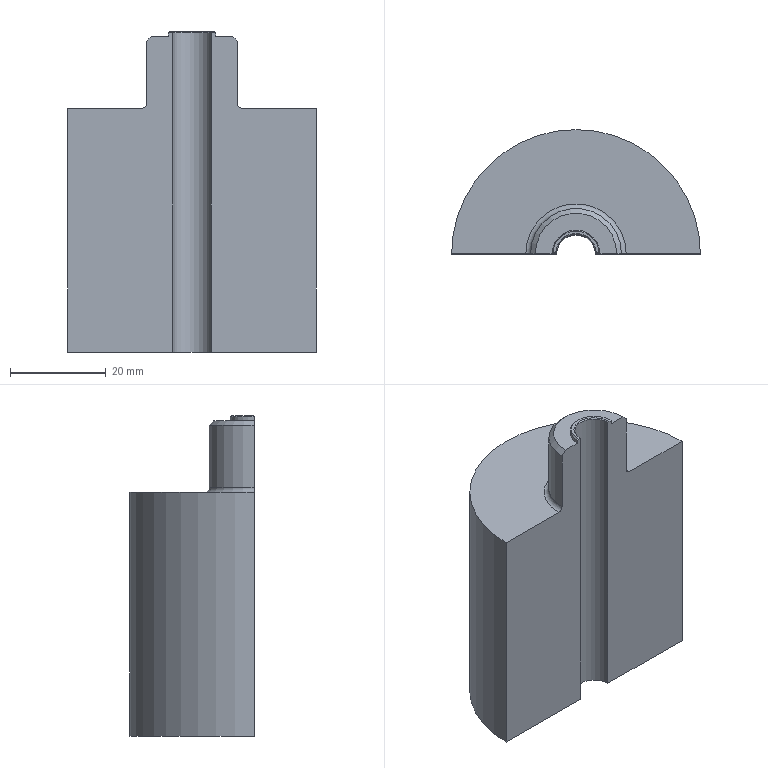Part | STEP file | 001-009-Riveting mechanism lower die insert | 1 solid | 16 faces | box 52 x 26 x 67 mm | volume 54586 mm3 | plane 8 | cylinder 4 | cone 3 | torus 1 | commonest cylinder face diameters 8.1 x1 10 x1 19 x1 52 x1
STEP:
#1=CARTESIAN_POINT('',(0.,0.,0.));
#2=DIRECTION('',(0.,0.,1.));
#3=DIRECTION('',(1.,0.,0.));
#4=AXIS2_PLACEMENT_3D('',#1,#2,#3);
#5=CARTESIAN_POINT('',(-5.,0.,66.));
#6=VERTEX_POINT('',#5);
#7=CARTESIAN_POINT('',(-8.5,0.,66.));
#8=VERTEX_POINT('',#7);
#9=CARTESIAN_POINT('',(0.,0.,66.));
#10=DIRECTION('',(-1.,0.,0.));
#11=VECTOR('',#10,1.);
#12=LINE('',#9,#11);
#13=CARTESIAN_POINT('',(0.,0.,0.));
#14=DIRECTION('',(0.,1.,0.));
#15=DIRECTION('',(0.,0.,1.));
#16=AXIS2_PLACEMENT_3D('',#13,#14,#15);
#17=PLANE('',#16);
#18=CARTESIAN_POINT('',(66.,0.));
#19=DIRECTION('',(0.,-1.));
#20=VECTOR('',#19,1.);
#21=LINE('',#18,#20);
#22=(GEOMETRIC_REPRESENTATION_CONTEXT(2)PARAMETRIC_REPRESENTATION_CONTEXT()REPRESENTATION_CONTEXT('',''));
#23=DEFINITIONAL_REPRESENTATION('',(#21),#22);
#24=PCURVE('',#17,#23);
#25=CARTESIAN_POINT('',(0.,0.,66.));
#26=DIRECTION('',(0.,0.,1.));
#27=DIRECTION('',(1.,0.,0.));
#28=AXIS2_PLACEMENT_3D('',#25,#26,#27);
#29=PLANE('',#28);
#30=CARTESIAN_POINT('',(0.,0.));
#31=DIRECTION('',(-1.,0.));
#32=VECTOR('',#31,1.);
#33=LINE('',#30,#32);
#34=(GEOMETRIC_REPRESENTATION_CONTEXT(2)PARAMETRIC_REPRESENTATION_CONTEXT()REPRESENTATION_CONTEXT('',''));
#35=DEFINITIONAL_REPRESENTATION('',(#33),#34);
#36=PCURVE('',#29,#35);
#37=SURFACE_CURVE('',#12,(#24,#36),.PCURVE_S1.);
#38=EDGE_CURVE('',#6,#8,#37,.T.);
#39=ORIENTED_EDGE('',*,*,#38,.T.);
#40=CARTESIAN_POINT('',(-9.5,0.,65.));
#41=VERTEX_POINT('',#40);
#42=CARTESIAN_POINT('',(0.,0.,74.5));
#43=DIRECTION('',(-0.7071,0.,-0.7071));
#44=VECTOR('',#43,1.);
#45=LINE('',#42,#44);
#46=CARTESIAN_POINT('',(74.5,0.));
#47=DIRECTION('',(-0.7071,-0.7071));
#48=VECTOR('',#47,1.);
#49=LINE('',#46,#48);
#50=(GEOMETRIC_REPRESENTATION_CONTEXT(2)PARAMETRIC_REPRESENTATION_CONTEXT()REPRESENTATION_CONTEXT('',''));
#51=DEFINITIONAL_REPRESENTATION('',(#49),#50);
#52=PCURVE('',#17,#51);
#53=CARTESIAN_POINT('',(0.,0.,66.));
#54=DIRECTION('',(0.,0.,-1.));
#55=DIRECTION('',(-1.,0.,0.));
#56=AXIS2_PLACEMENT_3D('',#53,#54,#55);
#57=CONICAL_SURFACE('',#56,8.5,0.7854);
#58=CARTESIAN_POINT('',(0.,-8.5));
#59=DIRECTION('',(0.,1.));
#60=VECTOR('',#59,1.);
#61=LINE('',#58,#60);
#62=(GEOMETRIC_REPRESENTATION_CONTEXT(2)PARAMETRIC_REPRESENTATION_CONTEXT()REPRESENTATION_CONTEXT('',''));
#63=DEFINITIONAL_REPRESENTATION('',(#61),#62);
#64=PCURVE('',#57,#63);
#65=SURFACE_CURVE('',#45,(#52,#64),.PCURVE_S1.);
#66=EDGE_CURVE('',#8,#41,#65,.T.);
#67=ORIENTED_EDGE('',*,*,#66,.T.);
#68=CARTESIAN_POINT('',(-9.5,0.,52.));
#69=VERTEX_POINT('',#68);
#70=CARTESIAN_POINT('',(-9.5,0.,67.));
#71=DIRECTION('',(0.,0.,1.));
#72=VECTOR('',#71,1.);
#73=LINE('',#70,#72);
#74=CARTESIAN_POINT('',(67.,-9.5));
#75=DIRECTION('',(1.,0.));
#76=VECTOR('',#75,1.);
#77=LINE('',#74,#76);
#78=(GEOMETRIC_REPRESENTATION_CONTEXT(2)PARAMETRIC_REPRESENTATION_CONTEXT()REPRESENTATION_CONTEXT('',''));
#79=DEFINITIONAL_REPRESENTATION('',(#77),#78);
#80=PCURVE('',#17,#79);
#81=CARTESIAN_POINT('',(0.,0.,67.));
#82=DIRECTION('',(0.,0.,-1.));
#83=DIRECTION('',(-1.,0.,0.));
#84=AXIS2_PLACEMENT_3D('',#81,#82,#83);
#85=CYLINDRICAL_SURFACE('',#84,9.5);
#86=CARTESIAN_POINT('',(0.,0.));
#87=DIRECTION('',(0.,-1.));
#88=VECTOR('',#87,1.);
#89=LINE('',#86,#88);
#90=(GEOMETRIC_REPRESENTATION_CONTEXT(2)PARAMETRIC_REPRESENTATION_CONTEXT()REPRESENTATION_CONTEXT('',''));
#91=DEFINITIONAL_REPRESENTATION('',(#89),#90);
#92=PCURVE('',#85,#91);
#93=SURFACE_CURVE('',#73,(#80,#92),.PCURVE_S1.);
#94=EDGE_CURVE('',#69,#41,#93,.T.);
#95=ORIENTED_EDGE('',*,*,#94,.F.);
#96=CARTESIAN_POINT('',(-10.5,0.,51.));
#97=VERTEX_POINT('',#96);
#98=CARTESIAN_POINT('',(-10.5,0.,52.));
#99=DIRECTION('',(0.,1.,0.));
#100=DIRECTION('',(0.,0.,1.));
#101=AXIS2_PLACEMENT_3D('',#98,#99,#100);
#102=CIRCLE('',#101,1.);
#103=CARTESIAN_POINT('',(52.,-10.5));
#104=DIRECTION('',(1.,0.));
#105=AXIS2_PLACEMENT_2D('',#103,#104);
#106=CIRCLE('',#105,1.);
#107=(GEOMETRIC_REPRESENTATION_CONTEXT(2)PARAMETRIC_REPRESENTATION_CONTEXT()REPRESENTATION_CONTEXT('',''));
#108=DEFINITIONAL_REPRESENTATION('',(#106),#107);
#109=PCURVE('',#17,#108);
#110=CARTESIAN_POINT('',(0.,0.,52.));
#111=DIRECTION('',(0.,0.,1.));
#112=DIRECTION('',(1.,0.,0.));
#113=AXIS2_PLACEMENT_3D('',#110,#111,#112);
#114=TOROIDAL_SURFACE('',#113,10.5,1.);
#115=CARTESIAN_POINT('',(3.142,1.571));
#116=DIRECTION('',(0.,1.));
#117=VECTOR('',#116,1.);
#118=LINE('',#115,#117);
#119=(GEOMETRIC_REPRESENTATION_CONTEXT(2)PARAMETRIC_REPRESENTATION_CONTEXT()REPRESENTATION_CONTEXT('',''));
#120=DEFINITIONAL_REPRESENTATION('',(#118),#119);
#121=PCURVE('',#114,#120);
#122=SURFACE_CURVE('',#102,(#109,#121),.PCURVE_S1.);
#123=EDGE_CURVE('',#69,#97,#122,.T.);
#124=ORIENTED_EDGE('',*,*,#123,.T.);
#125=CARTESIAN_POINT('',(-26.,0.,51.));
#126=VERTEX_POINT('',#125);
#127=CARTESIAN_POINT('',(0.,0.,51.));
#128=DIRECTION('',(-1.,0.,0.));
#129=VECTOR('',#128,1.);
#130=LINE('',#127,#129);
#131=CARTESIAN_POINT('',(51.,0.));
#132=DIRECTION('',(0.,-1.));
#133=VECTOR('',#132,1.);
#134=LINE('',#131,#133);
#135=(GEOMETRIC_REPRESENTATION_CONTEXT(2)PARAMETRIC_REPRESENTATION_CONTEXT()REPRESENTATION_CONTEXT('',''));
#136=DEFINITIONAL_REPRESENTATION('',(#134),#135);
#137=PCURVE('',#17,#136);
#138=CARTESIAN_POINT('',(0.,0.,51.));
#139=DIRECTION('',(0.,0.,1.));
#140=DIRECTION('',(1.,0.,0.));
#141=AXIS2_PLACEMENT_3D('',#138,#139,#140);
#142=PLANE('',#141);
#143=CARTESIAN_POINT('',(0.,0.));
#144=DIRECTION('',(-1.,0.));
#145=VECTOR('',#144,1.);
#146=LINE('',#143,#145);
#147=(GEOMETRIC_REPRESENTATION_CONTEXT(2)PARAMETRIC_REPRESENTATION_CONTEXT()REPRESENTATION_CONTEXT('',''));
#148=DEFINITIONAL_REPRESENTATION('',(#146),#147);
#149=PCURVE('',#142,#148);
#150=SURFACE_CURVE('',#130,(#137,#149),.PCURVE_S1.);
#151=EDGE_CURVE('',#97,#126,#150,.T.);
#152=ORIENTED_EDGE('',*,*,#151,.T.);
#153=CARTESIAN_POINT('',(-26.,0.,0.));
#154=VERTEX_POINT('',#153);
#155=CARTESIAN_POINT('',(-26.,0.,51.));
#156=DIRECTION('',(0.,0.,1.));
#157=VECTOR('',#156,1.);
#158=LINE('',#155,#157);
#159=CARTESIAN_POINT('',(51.,-26.));
#160=DIRECTION('',(1.,0.));
#161=VECTOR('',#160,1.);
#162=LINE('',#159,#161);
#163=(GEOMETRIC_REPRESENTATION_CONTEXT(2)PARAMETRIC_REPRESENTATION_CONTEXT()REPRESENTATION_CONTEXT('',''));
#164=DEFINITIONAL_REPRESENTATION('',(#162),#163);
#165=PCURVE('',#17,#164);
#166=CARTESIAN_POINT('',(0.,0.,51.));
#167=DIRECTION('',(0.,0.,-1.));
#168=DIRECTION('',(-1.,0.,0.));
#169=AXIS2_PLACEMENT_3D('',#166,#167,#168);
#170=CYLINDRICAL_SURFACE('',#169,26.);
#171=CARTESIAN_POINT('',(0.,0.));
#172=DIRECTION('',(0.,-1.));
#173=VECTOR('',#172,1.);
#174=LINE('',#171,#173);
#175=(GEOMETRIC_REPRESENTATION_CONTEXT(2)PARAMETRIC_REPRESENTATION_CONTEXT()REPRESENTATION_CONTEXT('',''));
#176=DEFINITIONAL_REPRESENTATION('',(#174),#175);
#177=PCURVE('',#170,#176);
#178=SURFACE_CURVE('',#158,(#165,#177),.PCURVE_S1.);
#179=EDGE_CURVE('',#154,#126,#178,.T.);
#180=ORIENTED_EDGE('',*,*,#179,.F.);
#181=CARTESIAN_POINT('',(-4.05,0.,0.));
#182=VERTEX_POINT('',#181);
#183=CARTESIAN_POINT('',(0.,0.,0.));
#184=DIRECTION('',(-1.,0.,0.));
#185=VECTOR('',#184,1.);
#186=LINE('',#183,#185);
#187=CARTESIAN_POINT('',(0.,0.));
#188=DIRECTION('',(0.,-1.));
#189=VECTOR('',#188,1.);
#190=LINE('',#187,#189);
#191=(GEOMETRIC_REPRESENTATION_CONTEXT(2)PARAMETRIC_REPRESENTATION_CONTEXT()REPRESENTATION_CONTEXT('',''));
#192=DEFINITIONAL_REPRESENTATION('',(#190),#191);
#193=PCURVE('',#17,#192);
#194=CARTESIAN_POINT('',(0.,0.,0.));
#195=DIRECTION('',(0.,0.,1.));
#196=DIRECTION('',(1.,0.,0.));
#197=AXIS2_PLACEMENT_3D('',#194,#195,#196);
#198=PLANE('',#197);
#199=CARTESIAN_POINT('',(0.,0.));
#200=DIRECTION('',(-1.,0.));
#201=VECTOR('',#200,1.);
#202=LINE('',#199,#201);
#203=(GEOMETRIC_REPRESENTATION_CONTEXT(2)PARAMETRIC_REPRESENTATION_CONTEXT()REPRESENTATION_CONTEXT('',''));
#204=DEFINITIONAL_REPRESENTATION('',(#202),#203);
#205=PCURVE('',#198,#204);
#206=SURFACE_CURVE('',#186,(#193,#205),.PCURVE_S1.);
#207=EDGE_CURVE('',#182,#154,#206,.T.);
#208=ORIENTED_EDGE('',*,*,#207,.F.);
#209=CARTESIAN_POINT('',(-4.05,0.,66.8));
#210=VERTEX_POINT('',#209);
#211=CARTESIAN_POINT('',(-4.05,0.,0.));
#212=DIRECTION('',(0.,0.,-1.));
#213=VECTOR('',#212,1.);
#214=LINE('',#211,#213);
#215=CARTESIAN_POINT('',(0.,-4.05));
#216=DIRECTION('',(-1.,0.));
#217=VECTOR('',#216,1.);
#218=LINE('',#215,#217);
#219=(GEOMETRIC_REPRESENTATION_CONTEXT(2)PARAMETRIC_REPRESENTATION_CONTEXT()REPRESENTATION_CONTEXT('',''));
#220=DEFINITIONAL_REPRESENTATION('',(#218),#219);
#221=PCURVE('',#17,#220);
#222=CARTESIAN_POINT('',(0.,0.,0.));
#223=DIRECTION('',(0.,0.,1.));
#224=DIRECTION('',(1.,0.,0.));
#225=AXIS2_PLACEMENT_3D('',#222,#223,#224);
#226=CYLINDRICAL_SURFACE('',#225,4.05);
#227=CARTESIAN_POINT('',(3.142,0.));
#228=DIRECTION('',(0.,-1.));
#229=VECTOR('',#228,1.);
#230=LINE('',#227,#229);
#231=(GEOMETRIC_REPRESENTATION_CONTEXT(2)PARAMETRIC_REPRESENTATION_CONTEXT()REPRESENTATION_CONTEXT('',''));
#232=DEFINITIONAL_REPRESENTATION('',(#230),#231);
#233=PCURVE('',#226,#232);
#234=SURFACE_CURVE('',#214,(#221,#233),.PCURVE_S1.);
#235=EDGE_CURVE('',#210,#182,#234,.T.);
#236=ORIENTED_EDGE('',*,*,#235,.F.);
#237=CARTESIAN_POINT('',(-5.,0.,66.8));
#238=VERTEX_POINT('',#237);
#239=CARTESIAN_POINT('',(-5.,0.,66.8));
#240=DIRECTION('',(-1.,0.,0.));
#241=VECTOR('',#240,1.);
#242=LINE('',#239,#241);
#243=CARTESIAN_POINT('',(66.8,-5.));
#244=DIRECTION('',(0.,-1.));
#245=VECTOR('',#244,1.);
#246=LINE('',#243,#245);
#247=(GEOMETRIC_REPRESENTATION_CONTEXT(2)PARAMETRIC_REPRESENTATION_CONTEXT()REPRESENTATION_CONTEXT('',''));
#248=DEFINITIONAL_REPRESENTATION('',(#246),#247);
#249=PCURVE('',#17,#248);
#250=CARTESIAN_POINT('',(0.,0.,66.8));
#251=DIRECTION('',(0.,-0.7071,0.7071));
#252=DIRECTION('',(1.,0.,0.));
#253=AXIS2_PLACEMENT_3D('',#250,#251,#252);
#254=PLANE('',#253);
#255=CARTESIAN_POINT('',(-5.,0.));
#256=DIRECTION('',(-1.,0.));
#257=VECTOR('',#256,1.);
#258=LINE('',#255,#257);
#259=(GEOMETRIC_REPRESENTATION_CONTEXT(2)PARAMETRIC_REPRESENTATION_CONTEXT()REPRESENTATION_CONTEXT('',''));
#260=DEFINITIONAL_REPRESENTATION('',(#258),#259);
#261=PCURVE('',#254,#260);
#262=SURFACE_CURVE('',#242,(#249,#261),.PCURVE_S1.);
#263=EDGE_CURVE('',#210,#238,#262,.T.);
#264=ORIENTED_EDGE('',*,*,#263,.T.);
#265=CARTESIAN_POINT('',(-5.,0.,66.));
#266=DIRECTION('',(0.,0.,-1.));
#267=VECTOR('',#266,1.);
#268=LINE('',#265,#267);
#269=CARTESIAN_POINT('',(66.,-5.));
#270=DIRECTION('',(-1.,0.));
#271=VECTOR('',#270,1.);
#272=LINE('',#269,#271);
#273=(GEOMETRIC_REPRESENTATION_CONTEXT(2)PARAMETRIC_REPRESENTATION_CONTEXT()REPRESENTATION_CONTEXT('',''));
#274=DEFINITIONAL_REPRESENTATION('',(#272),#273);
#275=PCURVE('',#17,#274);
#276=CARTESIAN_POINT('',(0.,0.,66.));
#277=DIRECTION('',(0.,0.,1.));
#278=DIRECTION('',(1.,0.,0.));
#279=AXIS2_PLACEMENT_3D('',#276,#277,#278);
#280=CYLINDRICAL_SURFACE('',#279,5.);
#281=CARTESIAN_POINT('',(3.142,0.));
#282=DIRECTION('',(0.,-1.));
#283=VECTOR('',#282,1.);
#284=LINE('',#281,#283);
#285=(GEOMETRIC_REPRESENTATION_CONTEXT(2)PARAMETRIC_REPRESENTATION_CONTEXT()REPRESENTATION_CONTEXT('',''));
#286=DEFINITIONAL_REPRESENTATION('',(#284),#285);
#287=PCURVE('',#280,#286);
#288=SURFACE_CURVE('',#268,(#275,#287),.PCURVE_S1.);
#289=EDGE_CURVE('',#238,#6,#288,.T.);
#290=ORIENTED_EDGE('',*,*,#289,.T.);
#291=EDGE_LOOP('',(#39,#67,#95,#124,#152,#180,#208,#236,#264,#290));
#292=FACE_BOUND('',#291,.T.);
#293=ADVANCED_FACE('',(#292),#17,.F.);
#294=ORIENTED_EDGE('',*,*,#94,.T.);
#295=CARTESIAN_POINT('',(9.5,0.,65.));
#296=VERTEX_POINT('',#295);
#297=CARTESIAN_POINT('',(0.,0.,65.));
#298=DIRECTION('',(0.,0.,-1.));
#299=DIRECTION('',(1.,0.,0.));
#300=AXIS2_PLACEMENT_3D('',#297,#298,#299);
#301=CIRCLE('',#300,9.5);
#302=CARTESIAN_POINT('',(-3.142,2.));
#303=DIRECTION('',(1.,0.));
#304=VECTOR('',#303,1.);
#305=LINE('',#302,#304);
#306=(GEOMETRIC_REPRESENTATION_CONTEXT(2)PARAMETRIC_REPRESENTATION_CONTEXT()REPRESENTATION_CONTEXT('',''));
#307=DEFINITIONAL_REPRESENTATION('',(#305),#306);
#308=PCURVE('',#85,#307);
#309=CARTESIAN_POINT('',(-3.142,1.));
#310=DIRECTION('',(1.,0.));
#311=VECTOR('',#310,1.);
#312=LINE('',#309,#311);
#313=(GEOMETRIC_REPRESENTATION_CONTEXT(2)PARAMETRIC_REPRESENTATION_CONTEXT()REPRESENTATION_CONTEXT('',''));
#314=DEFINITIONAL_REPRESENTATION('',(#312),#313);
#315=PCURVE('',#57,#314);
#316=SURFACE_CURVE('',#301,(#308,#315),.PCURVE_S1.);
#317=EDGE_CURVE('',#41,#296,#316,.T.);
#318=ORIENTED_EDGE('',*,*,#317,.T.);
#319=CARTESIAN_POINT('',(9.5,0.,52.));
#320=VERTEX_POINT('',#319);
#321=CARTESIAN_POINT('',(9.5,0.,67.));
#322=DIRECTION('',(0.,0.,-1.));
#323=VECTOR('',#322,1.);
#324=LINE('',#321,#323);
#325=CARTESIAN_POINT('',(3.142,0.));
#326=DIRECTION('',(0.,1.));
#327=VECTOR('',#326,1.);
#328=LINE('',#325,#327);
#329=(GEOMETRIC_REPRESENTATION_CONTEXT(2)PARAMETRIC_REPRESENTATION_CONTEXT()REPRESENTATION_CONTEXT('',''));
#330=DEFINITIONAL_REPRESENTATION('',(#328),#329);
#331=PCURVE('',#85,#330);
#332=CARTESIAN_POINT('',(0.,0.,0.));
#333=DIRECTION('',(0.,1.,0.));
#334=DIRECTION('',(0.,0.,1.));
#335=AXIS2_PLACEMENT_3D('',#332,#333,#334);
#336=PLANE('',#335);
#337=CARTESIAN_POINT('',(67.,9.5));
#338=DIRECTION('',(-1.,0.));
#339=VECTOR('',#338,1.);
#340=LINE('',#337,#339);
#341=(GEOMETRIC_REPRESENTATION_CONTEXT(2)PARAMETRIC_REPRESENTATION_CONTEXT()REPRESENTATION_CONTEXT('',''));
#342=DEFINITIONAL_REPRESENTATION('',(#340),#341);
#343=PCURVE('',#336,#342);
#344=SURFACE_CURVE('',#324,(#331,#343),.PCURVE_S1.);
#345=EDGE_CURVE('',#296,#320,#344,.T.);
#346=ORIENTED_EDGE('',*,*,#345,.T.);
#347=CARTESIAN_POINT('',(0.,0.,52.));
#348=DIRECTION('',(0.,0.,1.));
#349=DIRECTION('',(1.,0.,0.));
#350=AXIS2_PLACEMENT_3D('',#347,#348,#349);
#351=CIRCLE('',#350,9.5);
#352=CARTESIAN_POINT('',(3.142,15.));
#353=DIRECTION('',(-1.,0.));
#354=VECTOR('',#353,1.);
#355=LINE('',#352,#354);
#356=(GEOMETRIC_REPRESENTATION_CONTEXT(2)PARAMETRIC_REPRESENTATION_CONTEXT()REPRESENTATION_CONTEXT('',''));
#357=DEFINITIONAL_REPRESENTATION('',(#355),#356);
#358=PCURVE('',#85,#357);
#359=CARTESIAN_POINT('',(0.,3.142));
#360=DIRECTION('',(1.,0.));
#361=VECTOR('',#360,1.);
#362=LINE('',#359,#361);
#363=(GEOMETRIC_REPRESENTATION_CONTEXT(2)PARAMETRIC_REPRESENTATION_CONTEXT()REPRESENTATION_CONTEXT('',''));
#364=DEFINITIONAL_REPRESENTATION('',(#362),#363);
#365=PCURVE('',#114,#364);
#366=SURFACE_CURVE('',#351,(#358,#365),.PCURVE_S1.);
#367=EDGE_CURVE('',#320,#69,#366,.T.);
#368=ORIENTED_EDGE('',*,*,#367,.T.);
#369=EDGE_LOOP('',(#294,#318,#346,#368));
#370=FACE_BOUND('',#369,.T.);
#371=ADVANCED_FACE('',(#370),#85,.T.);
#372=CARTESIAN_POINT('',(-4.796,0.2,67.));
#373=VERTEX_POINT('',#372);
#374=CARTESIAN_POINT('',(-4.245,0.2,67.));
#375=VERTEX_POINT('',#374);
#376=CARTESIAN_POINT('',(-4.05,0.2,67.));
#377=DIRECTION('',(1.,0.,0.));
#378=VECTOR('',#377,1.);
#379=LINE('',#376,#378);
#380=CARTESIAN_POINT('',(0.,0.,67.));
#381=DIRECTION('',(0.,0.,1.));
#382=DIRECTION('',(1.,0.,0.));
#383=AXIS2_PLACEMENT_3D('',#380,#381,#382);
#384=PLANE('',#383);
#385=CARTESIAN_POINT('',(-4.05,0.2));
#386=DIRECTION('',(1.,0.));
#387=VECTOR('',#386,1.);
#388=LINE('',#385,#387);
#389=(GEOMETRIC_REPRESENTATION_CONTEXT(2)PARAMETRIC_REPRESENTATION_CONTEXT()REPRESENTATION_CONTEXT('',''));
#390=DEFINITIONAL_REPRESENTATION('',(#388),#389);
#391=PCURVE('',#384,#390);
#392=CARTESIAN_POINT('',(-4.05,0.2828));
#393=DIRECTION('',(1.,0.));
#394=VECTOR('',#393,1.);
#395=LINE('',#392,#394);
#396=(GEOMETRIC_REPRESENTATION_CONTEXT(2)PARAMETRIC_REPRESENTATION_CONTEXT()REPRESENTATION_CONTEXT('',''));
#397=DEFINITIONAL_REPRESENTATION('',(#395),#396);
#398=PCURVE('',#254,#397);
#399=SURFACE_CURVE('',#379,(#391,#398),.PCURVE_S1.);
#400=EDGE_CURVE('',#373,#375,#399,.T.);
#401=ORIENTED_EDGE('',*,*,#400,.T.);
#402=CARTESIAN_POINT('',(4.245,0.2,67.));
#403=VERTEX_POINT('',#402);
#404=CARTESIAN_POINT('',(0.,0.,67.));
#405=DIRECTION('',(0.,0.,-1.));
#406=DIRECTION('',(1.,0.,0.));
#407=AXIS2_PLACEMENT_3D('',#404,#405,#406);
#408=CIRCLE('',#407,4.25);
#409=CARTESIAN_POINT('',(4.25,0.));
#410=CARTESIAN_POINT('',(4.25,-7.361));
#411=CARTESIAN_POINT('',(-2.125,-3.681));
#412=CARTESIAN_POINT('',(-8.5,0.));
#413=CARTESIAN_POINT('',(-2.125,3.681));
#414=CARTESIAN_POINT('',(4.25,7.361));
#415=CARTESIAN_POINT('',(4.25,0.));
#416=(BOUNDED_CURVE()B_SPLINE_CURVE(2,(#409,#410,#411,#412,#413,#414,#415),.UNSPECIFIED.,.T.,.F.)B_SPLINE_CURVE_WITH_KNOTS((1,2,2,2,2,1),(-2.094,0.,2.094,4.189,6.283,8.378),.UNSPECIFIED.)CURVE()GEOMETRIC_REPRESENTATION_ITEM()RATIONAL_B_SPLINE_CURVE((1.,0.5,1.,0.5,1.,0.5,1.))REPRESENTATION_ITEM(''));
#417=(GEOMETRIC_REPRESENTATION_CONTEXT(2)PARAMETRIC_REPRESENTATION_CONTEXT()REPRESENTATION_CONTEXT('',''));
#418=DEFINITIONAL_REPRESENTATION('',(#416),#417);
#419=PCURVE('',#384,#418);
#420=CARTESIAN_POINT('',(0.,0.,66.8));
#421=DIRECTION('',(0.,0.,1.));
#422=DIRECTION('',(1.,0.,0.));
#423=AXIS2_PLACEMENT_3D('',#420,#421,#422);
#424=CONICAL_SURFACE('',#423,4.05,0.7854);
#425=CARTESIAN_POINT('',(6.283,0.2));
#426=DIRECTION('',(-1.,0.));
#427=VECTOR('',#426,1.);
#428=LINE('',#425,#427);
#429=(GEOMETRIC_REPRESENTATION_CONTEXT(2)PARAMETRIC_REPRESENTATION_CONTEXT()REPRESENTATION_CONTEXT('',''));
#430=DEFINITIONAL_REPRESENTATION('',(#428),#429);
#431=PCURVE('',#424,#430);
#432=SURFACE_CURVE('',#408,(#419,#431),.PCURVE_S1.);
#433=EDGE_CURVE('',#375,#403,#432,.T.);
#434=ORIENTED_EDGE('',*,*,#433,.T.);
#435=CARTESIAN_POINT('',(4.796,0.2,67.));
#436=VERTEX_POINT('',#435);
#437=CARTESIAN_POINT('',(5.,0.2,67.));
#438=DIRECTION('',(1.,0.,0.));
#439=VECTOR('',#438,1.);
#440=LINE('',#437,#439);
#441=CARTESIAN_POINT('',(5.,0.2));
#442=DIRECTION('',(1.,0.));
#443=VECTOR('',#442,1.);
#444=LINE('',#441,#443);
#445=(GEOMETRIC_REPRESENTATION_CONTEXT(2)PARAMETRIC_REPRESENTATION_CONTEXT()REPRESENTATION_CONTEXT('',''));
#446=DEFINITIONAL_REPRESENTATION('',(#444),#445);
#447=PCURVE('',#384,#446);
#448=CARTESIAN_POINT('',(0.,0.,66.8));
#449=DIRECTION('',(0.,-0.7071,0.7071));
#450=DIRECTION('',(1.,0.,0.));
#451=AXIS2_PLACEMENT_3D('',#448,#449,#450);
#452=PLANE('',#451);
#453=CARTESIAN_POINT('',(5.,0.2828));
#454=DIRECTION('',(1.,0.));
#455=VECTOR('',#454,1.);
#456=LINE('',#453,#455);
#457=(GEOMETRIC_REPRESENTATION_CONTEXT(2)PARAMETRIC_REPRESENTATION_CONTEXT()REPRESENTATION_CONTEXT('',''));
#458=DEFINITIONAL_REPRESENTATION('',(#456),#457);
#459=PCURVE('',#452,#458);
#460=SURFACE_CURVE('',#440,(#447,#459),.PCURVE_S1.);
#461=EDGE_CURVE('',#403,#436,#460,.T.);
#462=ORIENTED_EDGE('',*,*,#461,.T.);
#463=CARTESIAN_POINT('',(0.,0.,67.));
#464=DIRECTION('',(0.,0.,1.));
#465=DIRECTION('',(1.,0.,0.));
#466=AXIS2_PLACEMENT_3D('',#463,#464,#465);
#467=CIRCLE('',#466,4.8);
#468=CARTESIAN_POINT('',(0.,0.));
#469=DIRECTION('',(1.,0.));
#470=AXIS2_PLACEMENT_2D('',#468,#469);
#471=CIRCLE('',#470,4.8);
#472=(GEOMETRIC_REPRESENTATION_CONTEXT(2)PARAMETRIC_REPRESENTATION_CONTEXT()REPRESENTATION_CONTEXT('',''));
#473=DEFINITIONAL_REPRESENTATION('',(#471),#472);
#474=PCURVE('',#384,#473);
#475=CARTESIAN_POINT('',(0.,0.,67.));
#476=DIRECTION('',(0.,0.,-1.));
#477=DIRECTION('',(-1.,0.,0.));
#478=AXIS2_PLACEMENT_3D('',#475,#476,#477);
#479=CONICAL_SURFACE('',#478,4.8,0.7854);
#480=CARTESIAN_POINT('',(3.142,0.));
#481=DIRECTION('',(-1.,0.));
#482=VECTOR('',#481,1.);
#483=LINE('',#480,#482);
#484=(GEOMETRIC_REPRESENTATION_CONTEXT(2)PARAMETRIC_REPRESENTATION_CONTEXT()REPRESENTATION_CONTEXT('',''));
#485=DEFINITIONAL_REPRESENTATION('',(#483),#484);
#486=PCURVE('',#479,#485);
#487=SURFACE_CURVE('',#467,(#474,#486),.PCURVE_S1.);
#488=EDGE_CURVE('',#436,#373,#487,.T.);
#489=ORIENTED_EDGE('',*,*,#488,.T.);
#490=EDGE_LOOP('',(#401,#434,#462,#489));
#491=FACE_BOUND('',#490,.T.);
#492=ADVANCED_FACE('',(#491),#384,.T.);
#493=CARTESIAN_POINT('',(26.,0.,51.));
#494=VERTEX_POINT('',#493);
#495=CARTESIAN_POINT('',(0.,0.,51.));
#496=DIRECTION('',(0.,0.,1.));
#497=DIRECTION('',(1.,0.,0.));
#498=AXIS2_PLACEMENT_3D('',#495,#496,#497);
#499=CIRCLE('',#498,26.);
#500=CARTESIAN_POINT('',(3.142,0.));
#501=DIRECTION('',(-1.,0.));
#502=VECTOR('',#501,1.);
#503=LINE('',#500,#502);
#504=(GEOMETRIC_REPRESENTATION_CONTEXT(2)PARAMETRIC_REPRESENTATION_CONTEXT()REPRESENTATION_CONTEXT('',''));
#505=DEFINITIONAL_REPRESENTATION('',(#503),#504);
#506=PCURVE('',#170,#505);
#507=CARTESIAN_POINT('',(0.,0.));
#508=DIRECTION('',(1.,0.));
#509=AXIS2_PLACEMENT_2D('',#507,#508);
#510=CIRCLE('',#509,26.);
#511=(GEOMETRIC_REPRESENTATION_CONTEXT(2)PARAMETRIC_REPRESENTATION_CONTEXT()REPRESENTATION_CONTEXT('',''));
#512=DEFINITIONAL_REPRESENTATION('',(#510),#511);
#513=PCURVE('',#142,#512);
#514=SURFACE_CURVE('',#499,(#506,#513),.PCURVE_S1.);
#515=EDGE_CURVE('',#494,#126,#514,.T.);
#516=ORIENTED_EDGE('',*,*,#515,.F.);
#517=CARTESIAN_POINT('',(26.,0.,0.));
#518=VERTEX_POINT('',#517);
#519=CARTESIAN_POINT('',(26.,0.,51.));
#520=DIRECTION('',(0.,0.,-1.));
#521=VECTOR('',#520,1.);
#522=LINE('',#519,#521);
#523=CARTESIAN_POINT('',(3.142,0.));
#524=DIRECTION('',(0.,1.));
#525=VECTOR('',#524,1.);
#526=LINE('',#523,#525);
#527=(GEOMETRIC_REPRESENTATION_CONTEXT(2)PARAMETRIC_REPRESENTATION_CONTEXT()REPRESENTATION_CONTEXT('',''));
#528=DEFINITIONAL_REPRESENTATION('',(#526),#527);
#529=PCURVE('',#170,#528);
#530=CARTESIAN_POINT('',(51.,26.));
#531=DIRECTION('',(-1.,0.));
#532=VECTOR('',#531,1.);
#533=LINE('',#530,#532);
#534=(GEOMETRIC_REPRESENTATION_CONTEXT(2)PARAMETRIC_REPRESENTATION_CONTEXT()REPRESENTATION_CONTEXT('',''));
#535=DEFINITIONAL_REPRESENTATION('',(#533),#534);
#536=PCURVE('',#336,#535);
#537=SURFACE_CURVE('',#522,(#529,#536),.PCURVE_S1.);
#538=EDGE_CURVE('',#494,#518,#537,.T.);
#539=ORIENTED_EDGE('',*,*,#538,.T.);
#540=CARTESIAN_POINT('',(0.,0.,0.));
#541=DIRECTION('',(0.,0.,1.));
#542=DIRECTION('',(1.,0.,0.));
#543=AXIS2_PLACEMENT_3D('',#540,#541,#542);
#544=CIRCLE('',#543,26.);
#545=CARTESIAN_POINT('',(3.142,51.));
#546=DIRECTION('',(-1.,0.));
#547=VECTOR('',#546,1.);
#548=LINE('',#545,#547);
#549=(GEOMETRIC_REPRESENTATION_CONTEXT(2)PARAMETRIC_REPRESENTATION_CONTEXT()REPRESENTATION_CONTEXT('',''));
#550=DEFINITIONAL_REPRESENTATION('',(#548),#549);
#551=PCURVE('',#170,#550);
#552=CARTESIAN_POINT('',(0.,0.));
#553=DIRECTION('',(1.,0.));
#554=AXIS2_PLACEMENT_2D('',#552,#553);
#555=CIRCLE('',#554,26.);
#556=(GEOMETRIC_REPRESENTATION_CONTEXT(2)PARAMETRIC_REPRESENTATION_CONTEXT()REPRESENTATION_CONTEXT('',''));
#557=DEFINITIONAL_REPRESENTATION('',(#555),#556);
#558=PCURVE('',#198,#557);
#559=SURFACE_CURVE('',#544,(#551,#558),.PCURVE_S1.);
#560=EDGE_CURVE('',#518,#154,#559,.T.);
#561=ORIENTED_EDGE('',*,*,#560,.T.);
#562=ORIENTED_EDGE('',*,*,#179,.T.);
#563=EDGE_LOOP('',(#516,#539,#561,#562));
#564=FACE_BOUND('',#563,.T.);
#565=ADVANCED_FACE('',(#564),#170,.T.);
#566=ORIENTED_EDGE('',*,*,#151,.F.);
#567=CARTESIAN_POINT('',(10.5,0.,51.));
#568=VERTEX_POINT('',#567);
#569=CARTESIAN_POINT('',(0.,0.,51.));
#570=DIRECTION('',(0.,0.,-1.));
#571=DIRECTION('',(1.,0.,0.));
#572=AXIS2_PLACEMENT_3D('',#569,#570,#571);
#573=CIRCLE('',#572,10.5);
#574=CARTESIAN_POINT('',(10.5,0.));
#575=CARTESIAN_POINT('',(10.5,-18.187));
#576=CARTESIAN_POINT('',(-5.25,-9.093));
#577=CARTESIAN_POINT('',(-21.,0.));
#578=CARTESIAN_POINT('',(-5.25,9.093));
#579=CARTESIAN_POINT('',(10.5,18.187));
#580=CARTESIAN_POINT('',(10.5,0.));
#581=(BOUNDED_CURVE()B_SPLINE_CURVE(2,(#574,#575,#576,#577,#578,#579,#580),.UNSPECIFIED.,.T.,.F.)B_SPLINE_CURVE_WITH_KNOTS((1,2,2,2,2,1),(-2.094,0.,2.094,4.189,6.283,8.378),.UNSPECIFIED.)CURVE()GEOMETRIC_REPRESENTATION_ITEM()RATIONAL_B_SPLINE_CURVE((1.,0.5,1.,0.5,1.,0.5,1.))REPRESENTATION_ITEM(''));
#582=(GEOMETRIC_REPRESENTATION_CONTEXT(2)PARAMETRIC_REPRESENTATION_CONTEXT()REPRESENTATION_CONTEXT('',''));
#583=DEFINITIONAL_REPRESENTATION('',(#581),#582);
#584=PCURVE('',#142,#583);
#585=CARTESIAN_POINT('',(6.283,4.712));
#586=DIRECTION('',(-1.,0.));
#587=VECTOR('',#586,1.);
#588=LINE('',#585,#587);
#589=(GEOMETRIC_REPRESENTATION_CONTEXT(2)PARAMETRIC_REPRESENTATION_CONTEXT()REPRESENTATION_CONTEXT('',''));
#590=DEFINITIONAL_REPRESENTATION('',(#588),#589);
#591=PCURVE('',#114,#590);
#592=SURFACE_CURVE('',#573,(#584,#591),.PCURVE_S1.);
#593=EDGE_CURVE('',#97,#568,#592,.T.);
#594=ORIENTED_EDGE('',*,*,#593,.T.);
#595=CARTESIAN_POINT('',(0.,0.,51.));
#596=DIRECTION('',(-1.,0.,0.));
#597=VECTOR('',#596,1.);
#598=LINE('',#595,#597);
#599=CARTESIAN_POINT('',(0.,0.));
#600=DIRECTION('',(-1.,0.));
#601=VECTOR('',#600,1.);
#602=LINE('',#599,#601);
#603=(GEOMETRIC_REPRESENTATION_CONTEXT(2)PARAMETRIC_REPRESENTATION_CONTEXT()REPRESENTATION_CONTEXT('',''));
#604=DEFINITIONAL_REPRESENTATION('',(#602),#603);
#605=PCURVE('',#142,#604);
#606=CARTESIAN_POINT('',(51.,0.));
#607=DIRECTION('',(0.,-1.));
#608=VECTOR('',#607,1.);
#609=LINE('',#606,#608);
#610=(GEOMETRIC_REPRESENTATION_CONTEXT(2)PARAMETRIC_REPRESENTATION_CONTEXT()REPRESENTATION_CONTEXT('',''));
#611=DEFINITIONAL_REPRESENTATION('',(#609),#610);
#612=PCURVE('',#336,#611);
#613=SURFACE_CURVE('',#598,(#605,#612),.PCURVE_S1.);
#614=EDGE_CURVE('',#494,#568,#613,.T.);
#615=ORIENTED_EDGE('',*,*,#614,.F.);
#616=ORIENTED_EDGE('',*,*,#515,.T.);
#617=EDGE_LOOP('',(#566,#594,#615,#616));
#618=FACE_BOUND('',#617,.T.);
#619=ADVANCED_FACE('',(#618),#142,.T.);
#620=ORIENTED_EDGE('',*,*,#560,.F.);
#621=CARTESIAN_POINT('',(4.05,0.,0.));
#622=VERTEX_POINT('',#621);
#623=CARTESIAN_POINT('',(0.,0.,0.));
#624=DIRECTION('',(-1.,0.,0.));
#625=VECTOR('',#624,1.);
#626=LINE('',#623,#625);
#627=CARTESIAN_POINT('',(0.,0.));
#628=DIRECTION('',(-1.,0.));
#629=VECTOR('',#628,1.);
#630=LINE('',#627,#629);
#631=(GEOMETRIC_REPRESENTATION_CONTEXT(2)PARAMETRIC_REPRESENTATION_CONTEXT()REPRESENTATION_CONTEXT('',''));
#632=DEFINITIONAL_REPRESENTATION('',(#630),#631);
#633=PCURVE('',#198,#632);
#634=CARTESIAN_POINT('',(0.,0.));
#635=DIRECTION('',(0.,-1.));
#636=VECTOR('',#635,1.);
#637=LINE('',#634,#636);
#638=(GEOMETRIC_REPRESENTATION_CONTEXT(2)PARAMETRIC_REPRESENTATION_CONTEXT()REPRESENTATION_CONTEXT('',''));
#639=DEFINITIONAL_REPRESENTATION('',(#637),#638);
#640=PCURVE('',#336,#639);
#641=SURFACE_CURVE('',#626,(#633,#640),.PCURVE_S1.);
#642=EDGE_CURVE('',#518,#622,#641,.T.);
#643=ORIENTED_EDGE('',*,*,#642,.T.);
#644=CARTESIAN_POINT('',(0.,0.,0.));
#645=DIRECTION('',(0.,0.,1.));
#646=DIRECTION('',(1.,0.,0.));
#647=AXIS2_PLACEMENT_3D('',#644,#645,#646);
#648=CIRCLE('',#647,4.05);
#649=CARTESIAN_POINT('',(0.,0.));
#650=DIRECTION('',(1.,0.));
#651=AXIS2_PLACEMENT_2D('',#649,#650);
#652=CIRCLE('',#651,4.05);
#653=(GEOMETRIC_REPRESENTATION_CONTEXT(2)PARAMETRIC_REPRESENTATION_CONTEXT()REPRESENTATION_CONTEXT('',''));
#654=DEFINITIONAL_REPRESENTATION('',(#652),#653);
#655=PCURVE('',#198,#654);
#656=CARTESIAN_POINT('',(0.,0.));
#657=DIRECTION('',(1.,0.));
#658=VECTOR('',#657,1.);
#659=LINE('',#656,#658);
#660=(GEOMETRIC_REPRESENTATION_CONTEXT(2)PARAMETRIC_REPRESENTATION_CONTEXT()REPRESENTATION_CONTEXT('',''));
#661=DEFINITIONAL_REPRESENTATION('',(#659),#660);
#662=PCURVE('',#226,#661);
#663=SURFACE_CURVE('',#648,(#655,#662),.PCURVE_S1.);
#664=EDGE_CURVE('',#622,#182,#663,.T.);
#665=ORIENTED_EDGE('',*,*,#664,.T.);
#666=ORIENTED_EDGE('',*,*,#207,.T.);
#667=EDGE_LOOP('',(#620,#643,#665,#666));
#668=FACE_BOUND('',#667,.T.);
#669=ADVANCED_FACE('',(#668),#198,.F.);
#670=ORIENTED_EDGE('',*,*,#664,.T.);
#671=ORIENTED_EDGE('',*,*,#235,.F.);
#672=CARTESIAN_POINT('',(4.05,0.,66.8));
#673=VERTEX_POINT('',#672);
#674=CARTESIAN_POINT('',(0.,0.,66.8));
#675=DIRECTION('',(0.,0.,1.));
#676=DIRECTION('',(1.,0.,0.));
#677=AXIS2_PLACEMENT_3D('',#674,#675,#676);
#678=CIRCLE('',#677,4.05);
#679=CARTESIAN_POINT('',(0.,66.8));
#680=DIRECTION('',(1.,0.));
#681=VECTOR('',#680,1.);
#682=LINE('',#679,#681);
#683=(GEOMETRIC_REPRESENTATION_CONTEXT(2)PARAMETRIC_REPRESENTATION_CONTEXT()REPRESENTATION_CONTEXT('',''));
#684=DEFINITIONAL_REPRESENTATION('',(#682),#683);
#685=PCURVE('',#226,#684);
#686=CARTESIAN_POINT('',(0.,0.));
#687=DIRECTION('',(1.,0.));
#688=VECTOR('',#687,1.);
#689=LINE('',#686,#688);
#690=(GEOMETRIC_REPRESENTATION_CONTEXT(2)PARAMETRIC_REPRESENTATION_CONTEXT()REPRESENTATION_CONTEXT('',''));
#691=DEFINITIONAL_REPRESENTATION('',(#689),#690);
#692=PCURVE('',#424,#691);
#693=SURFACE_CURVE('',#678,(#685,#692),.PCURVE_S1.);
#694=EDGE_CURVE('',#673,#210,#693,.T.);
#695=ORIENTED_EDGE('',*,*,#694,.F.);
#696=CARTESIAN_POINT('',(4.05,0.,0.));
#697=DIRECTION('',(0.,0.,1.));
#698=VECTOR('',#697,1.);
#699=LINE('',#696,#698);
#700=CARTESIAN_POINT('',(0.,0.));
#701=DIRECTION('',(0.,1.));
#702=VECTOR('',#701,1.);
#703=LINE('',#700,#702);
#704=(GEOMETRIC_REPRESENTATION_CONTEXT(2)PARAMETRIC_REPRESENTATION_CONTEXT()REPRESENTATION_CONTEXT('',''));
#705=DEFINITIONAL_REPRESENTATION('',(#703),#704);
#706=PCURVE('',#226,#705);
#707=CARTESIAN_POINT('',(0.,4.05));
#708=DIRECTION('',(1.,0.));
#709=VECTOR('',#708,1.);
#710=LINE('',#707,#709);
#711=(GEOMETRIC_REPRESENTATION_CONTEXT(2)PARAMETRIC_REPRESENTATION_CONTEXT()REPRESENTATION_CONTEXT('',''));
#712=DEFINITIONAL_REPRESENTATION('',(#710),#711);
#713=PCURVE('',#336,#712);
#714=SURFACE_CURVE('',#699,(#706,#713),.PCURVE_S1.);
#715=EDGE_CURVE('',#622,#673,#714,.T.);
#716=ORIENTED_EDGE('',*,*,#715,.F.);
#717=EDGE_LOOP('',(#670,#671,#695,#716));
#718=FACE_BOUND('',#717,.F.);
#719=ADVANCED_FACE('',(#718),#226,.F.);
#720=CARTESIAN_POINT('',(8.5,0.,66.));
#721=VERTEX_POINT('',#720);
#722=CARTESIAN_POINT('',(5.,0.,66.));
#723=VERTEX_POINT('',#722);
#724=CARTESIAN_POINT('',(0.,0.,66.));
#725=DIRECTION('',(-1.,0.,0.));
#726=VECTOR('',#725,1.);
#727=LINE('',#724,#726);
#728=CARTESIAN_POINT('',(0.,0.));
#729=DIRECTION('',(-1.,0.));
#730=VECTOR('',#729,1.);
#731=LINE('',#728,#730);
#732=(GEOMETRIC_REPRESENTATION_CONTEXT(2)PARAMETRIC_REPRESENTATION_CONTEXT()REPRESENTATION_CONTEXT('',''));
#733=DEFINITIONAL_REPRESENTATION('',(#731),#732);
#734=PCURVE('',#29,#733);
#735=CARTESIAN_POINT('',(66.,0.));
#736=DIRECTION('',(0.,-1.));
#737=VECTOR('',#736,1.);
#738=LINE('',#735,#737);
#739=(GEOMETRIC_REPRESENTATION_CONTEXT(2)PARAMETRIC_REPRESENTATION_CONTEXT()REPRESENTATION_CONTEXT('',''));
#740=DEFINITIONAL_REPRESENTATION('',(#738),#739);
#741=PCURVE('',#336,#740);
#742=SURFACE_CURVE('',#727,(#734,#741),.PCURVE_S1.);
#743=EDGE_CURVE('',#721,#723,#742,.T.);
#744=ORIENTED_EDGE('',*,*,#743,.F.);
#745=CARTESIAN_POINT('',(0.,0.,66.));
#746=DIRECTION('',(0.,0.,1.));
#747=DIRECTION('',(1.,0.,0.));
#748=AXIS2_PLACEMENT_3D('',#745,#746,#747);
#749=CIRCLE('',#748,8.5);
#750=CARTESIAN_POINT('',(0.,0.));
#751=DIRECTION('',(1.,0.));
#752=AXIS2_PLACEMENT_2D('',#750,#751);
#753=CIRCLE('',#752,8.5);
#754=(GEOMETRIC_REPRESENTATION_CONTEXT(2)PARAMETRIC_REPRESENTATION_CONTEXT()REPRESENTATION_CONTEXT('',''));
#755=DEFINITIONAL_REPRESENTATION('',(#753),#754);
#756=PCURVE('',#29,#755);
#757=CARTESIAN_POINT('',(3.142,0.));
#758=DIRECTION('',(-1.,0.));
#759=VECTOR('',#758,1.);
#760=LINE('',#757,#759);
#761=(GEOMETRIC_REPRESENTATION_CONTEXT(2)PARAMETRIC_REPRESENTATION_CONTEXT()REPRESENTATION_CONTEXT('',''));
#762=DEFINITIONAL_REPRESENTATION('',(#760),#761);
#763=PCURVE('',#57,#762);
#764=SURFACE_CURVE('',#749,(#756,#763),.PCURVE_S1.);
#765=EDGE_CURVE('',#721,#8,#764,.T.);
#766=ORIENTED_EDGE('',*,*,#765,.T.);
#767=ORIENTED_EDGE('',*,*,#38,.F.);
#768=CARTESIAN_POINT('',(0.,0.,66.));
#769=DIRECTION('',(0.,0.,1.));
#770=DIRECTION('',(1.,0.,0.));
#771=AXIS2_PLACEMENT_3D('',#768,#769,#770);
#772=CIRCLE('',#771,5.);
#773=CARTESIAN_POINT('',(0.,0.));
#774=DIRECTION('',(1.,0.));
#775=AXIS2_PLACEMENT_2D('',#773,#774);
#776=CIRCLE('',#775,5.);
#777=(GEOMETRIC_REPRESENTATION_CONTEXT(2)PARAMETRIC_REPRESENTATION_CONTEXT()REPRESENTATION_CONTEXT('',''));
#778=DEFINITIONAL_REPRESENTATION('',(#776),#777);
#779=PCURVE('',#29,#778);
#780=CARTESIAN_POINT('',(0.,0.));
#781=DIRECTION('',(1.,0.));
#782=VECTOR('',#781,1.);
#783=LINE('',#780,#782);
#784=(GEOMETRIC_REPRESENTATION_CONTEXT(2)PARAMETRIC_REPRESENTATION_CONTEXT()REPRESENTATION_CONTEXT('',''));
#785=DEFINITIONAL_REPRESENTATION('',(#783),#784);
#786=PCURVE('',#280,#785);
#787=SURFACE_CURVE('',#772,(#779,#786),.PCURVE_S1.);
#788=EDGE_CURVE('',#723,#6,#787,.T.);
#789=ORIENTED_EDGE('',*,*,#788,.F.);
#790=EDGE_LOOP('',(#744,#766,#767,#789));
#791=FACE_BOUND('',#790,.T.);
#792=ADVANCED_FACE('',(#791),#29,.T.);
#793=ORIENTED_EDGE('',*,*,#289,.F.);
#794=CARTESIAN_POINT('',(5.,0.,66.8));
#795=VERTEX_POINT('',#794);
#796=CARTESIAN_POINT('',(0.,0.,66.8));
#797=DIRECTION('',(0.,0.,-1.));
#798=DIRECTION('',(1.,0.,0.));
#799=AXIS2_PLACEMENT_3D('',#796,#797,#798);
#800=CIRCLE('',#799,5.);
#801=CARTESIAN_POINT('',(6.283,0.8));
#802=DIRECTION('',(-1.,0.));
#803=VECTOR('',#802,1.);
#804=LINE('',#801,#803);
#805=(GEOMETRIC_REPRESENTATION_CONTEXT(2)PARAMETRIC_REPRESENTATION_CONTEXT()REPRESENTATION_CONTEXT('',''));
#806=DEFINITIONAL_REPRESENTATION('',(#804),#805);
#807=PCURVE('',#280,#806);
#808=CARTESIAN_POINT('',(-3.142,0.2));
#809=DIRECTION('',(1.,0.));
#810=VECTOR('',#809,1.);
#811=LINE('',#808,#810);
#812=(GEOMETRIC_REPRESENTATION_CONTEXT(2)PARAMETRIC_REPRESENTATION_CONTEXT()REPRESENTATION_CONTEXT('',''));
#813=DEFINITIONAL_REPRESENTATION('',(#811),#812);
#814=PCURVE('',#479,#813);
#815=SURFACE_CURVE('',#800,(#807,#814),.PCURVE_S1.);
#816=EDGE_CURVE('',#238,#795,#815,.T.);
#817=ORIENTED_EDGE('',*,*,#816,.T.);
#818=CARTESIAN_POINT('',(5.,0.,66.));
#819=DIRECTION('',(0.,0.,1.));
#820=VECTOR('',#819,1.);
#821=LINE('',#818,#820);
#822=CARTESIAN_POINT('',(0.,0.));
#823=DIRECTION('',(0.,1.));
#824=VECTOR('',#823,1.);
#825=LINE('',#822,#824);
#826=(GEOMETRIC_REPRESENTATION_CONTEXT(2)PARAMETRIC_REPRESENTATION_CONTEXT()REPRESENTATION_CONTEXT('',''));
#827=DEFINITIONAL_REPRESENTATION('',(#825),#826);
#828=PCURVE('',#280,#827);
#829=CARTESIAN_POINT('',(66.,5.));
#830=DIRECTION('',(1.,0.));
#831=VECTOR('',#830,1.);
#832=LINE('',#829,#831);
#833=(GEOMETRIC_REPRESENTATION_CONTEXT(2)PARAMETRIC_REPRESENTATION_CONTEXT()REPRESENTATION_CONTEXT('',''));
#834=DEFINITIONAL_REPRESENTATION('',(#832),#833);
#835=PCURVE('',#336,#834);
#836=SURFACE_CURVE('',#821,(#828,#835),.PCURVE_S1.);
#837=EDGE_CURVE('',#723,#795,#836,.T.);
#838=ORIENTED_EDGE('',*,*,#837,.F.);
#839=ORIENTED_EDGE('',*,*,#788,.T.);
#840=EDGE_LOOP('',(#793,#817,#838,#839));
#841=FACE_BOUND('',#840,.T.);
#842=ADVANCED_FACE('',(#841),#280,.T.);
#843=ORIENTED_EDGE('',*,*,#345,.F.);
#844=CARTESIAN_POINT('',(0.,0.,74.5));
#845=DIRECTION('',(-0.7071,0.,0.7071));
#846=VECTOR('',#845,1.);
#847=LINE('',#844,#846);
#848=CARTESIAN_POINT('',(74.5,0.));
#849=DIRECTION('',(0.7071,-0.7071));
#850=VECTOR('',#849,1.);
#851=LINE('',#848,#850);
#852=(GEOMETRIC_REPRESENTATION_CONTEXT(2)PARAMETRIC_REPRESENTATION_CONTEXT()REPRESENTATION_CONTEXT('',''));
#853=DEFINITIONAL_REPRESENTATION('',(#851),#852);
#854=PCURVE('',#336,#853);
#855=CARTESIAN_POINT('',(3.142,-8.5));
#856=DIRECTION('',(0.,-1.));
#857=VECTOR('',#856,1.);
#858=LINE('',#855,#857);
#859=(GEOMETRIC_REPRESENTATION_CONTEXT(2)PARAMETRIC_REPRESENTATION_CONTEXT()REPRESENTATION_CONTEXT('',''));
#860=DEFINITIONAL_REPRESENTATION('',(#858),#859);
#861=PCURVE('',#57,#860);
#862=SURFACE_CURVE('',#847,(#854,#861),.PCURVE_S1.);
#863=EDGE_CURVE('',#296,#721,#862,.T.);
#864=ORIENTED_EDGE('',*,*,#863,.T.);
#865=ORIENTED_EDGE('',*,*,#743,.T.);
#866=ORIENTED_EDGE('',*,*,#837,.T.);
#867=CARTESIAN_POINT('',(4.05,0.,66.8));
#868=DIRECTION('',(-1.,0.,0.));
#869=VECTOR('',#868,1.);
#870=LINE('',#867,#869);
#871=CARTESIAN_POINT('',(66.8,4.05));
#872=DIRECTION('',(0.,-1.));
#873=VECTOR('',#872,1.);
#874=LINE('',#871,#873);
#875=(GEOMETRIC_REPRESENTATION_CONTEXT(2)PARAMETRIC_REPRESENTATION_CONTEXT()REPRESENTATION_CONTEXT('',''));
#876=DEFINITIONAL_REPRESENTATION('',(#874),#875);
#877=PCURVE('',#336,#876);
#878=CARTESIAN_POINT('',(4.05,0.));
#879=DIRECTION('',(-1.,0.));
#880=VECTOR('',#879,1.);
#881=LINE('',#878,#880);
#882=(GEOMETRIC_REPRESENTATION_CONTEXT(2)PARAMETRIC_REPRESENTATION_CONTEXT()REPRESENTATION_CONTEXT('',''));
#883=DEFINITIONAL_REPRESENTATION('',(#881),#882);
#884=PCURVE('',#452,#883);
#885=SURFACE_CURVE('',#870,(#877,#884),.PCURVE_S1.);
#886=EDGE_CURVE('',#795,#673,#885,.T.);
#887=ORIENTED_EDGE('',*,*,#886,.T.);
#888=ORIENTED_EDGE('',*,*,#715,.F.);
#889=ORIENTED_EDGE('',*,*,#642,.F.);
#890=ORIENTED_EDGE('',*,*,#538,.F.);
#891=ORIENTED_EDGE('',*,*,#614,.T.);
#892=CARTESIAN_POINT('',(10.5,0.,52.));
#893=DIRECTION('',(0.,1.,0.));
#894=DIRECTION('',(0.,0.,1.));
#895=AXIS2_PLACEMENT_3D('',#892,#893,#894);
#896=CIRCLE('',#895,1.);
#897=CARTESIAN_POINT('',(52.,10.5));
#898=DIRECTION('',(1.,0.));
#899=AXIS2_PLACEMENT_2D('',#897,#898);
#900=CIRCLE('',#899,1.);
#901=(GEOMETRIC_REPRESENTATION_CONTEXT(2)PARAMETRIC_REPRESENTATION_CONTEXT()REPRESENTATION_CONTEXT('',''));
#902=DEFINITIONAL_REPRESENTATION('',(#900),#901);
#903=PCURVE('',#336,#902);
#904=CARTESIAN_POINT('',(0.,7.854));
#905=DIRECTION('',(0.,-1.));
#906=VECTOR('',#905,1.);
#907=LINE('',#904,#906);
#908=(GEOMETRIC_REPRESENTATION_CONTEXT(2)PARAMETRIC_REPRESENTATION_CONTEXT()REPRESENTATION_CONTEXT('',''));
#909=DEFINITIONAL_REPRESENTATION('',(#907),#908);
#910=PCURVE('',#114,#909);
#911=SURFACE_CURVE('',#896,(#903,#910),.PCURVE_S1.);
#912=EDGE_CURVE('',#568,#320,#911,.T.);
#913=ORIENTED_EDGE('',*,*,#912,.T.);
#914=EDGE_LOOP('',(#843,#864,#865,#866,#887,#888,#889,#890,#891,#913));
#915=FACE_BOUND('',#914,.T.);
#916=ADVANCED_FACE('',(#915),#336,.F.);
#917=CARTESIAN_POINT('',(-4.796,0.2,67.));
#918=CARTESIAN_POINT('',(-4.865,0.1338,66.934));
#919=CARTESIAN_POINT('',(-4.933,0.06713,66.867));
#920=CARTESIAN_POINT('',(-5.,0.,66.8));
#921=B_SPLINE_CURVE_WITH_KNOTS('',3,(#917,#918,#919,#920),.UNSPECIFIED.,.F.,.F.,(4,4),(0.,0.0003488),.PIECEWISE_BEZIER_KNOTS.);
#922=CARTESIAN_POINT('',(0.04168,0.));
#923=CARTESIAN_POINT('',(0.04103,0.003008));
#924=CARTESIAN_POINT('',(0.03972,0.009027));
#925=CARTESIAN_POINT('',(0.03777,0.01806));
#926=CARTESIAN_POINT('',(0.03582,0.0271));
#927=CARTESIAN_POINT('',(0.03389,0.03615));
#928=CARTESIAN_POINT('',(0.03195,0.0452));
#929=CARTESIAN_POINT('',(0.03003,0.05426));
#930=CARTESIAN_POINT('',(0.02811,0.06332));
#931=CARTESIAN_POINT('',(0.02619,0.07239));
#932=CARTESIAN_POINT('',(0.02428,0.08147));
#933=CARTESIAN_POINT('',(0.02238,0.09055));
#934=CARTESIAN_POINT('',(0.02048,0.09964));
#935=CARTESIAN_POINT('',(0.01859,0.1087));
#936=CARTESIAN_POINT('',(0.01671,0.1178));
#937=CARTESIAN_POINT('',(0.01483,0.1269));
#938=CARTESIAN_POINT('',(0.01295,0.1361));
#939=CARTESIAN_POINT('',(0.01109,0.1452));
#940=CARTESIAN_POINT('',(0.009224,0.1543));
#941=CARTESIAN_POINT('',(0.007368,0.1634));
#942=CARTESIAN_POINT('',(0.005517,0.1726));
#943=CARTESIAN_POINT('',(0.003672,0.1817));
#944=CARTESIAN_POINT('',(0.001833,0.1908));
#945=CARTESIAN_POINT('',(0.0006103,0.1969));
#946=CARTESIAN_POINT('',(0.,0.2));
#947=B_SPLINE_CURVE_WITH_KNOTS('',3,(#922,#923,#924,#925,#926,#927,#928,#929,#930,#931,#932,#933,#934,#935,#936,#937,#938,#939,#940,#941,#942,#943,#944,#945,#946),.UNSPECIFIED.,.F.,.F.,(4,1,1,1,1,1,1,1,1,1,1,1,1,1,1,1,1,1,1,1,1,1,4),(0.,0.00001586,0.00003171,0.00004757,0.00006342,0.00007928,0.00009514,0.000111,0.0001268,0.0001427,0.0001586,0.0001744,0.0001903,0.0002061,0.000222,0.0002378,0.0002537,0.0002696,0.0002854,0.0003013,0.0003171,0.000333,0.0003488),.QUASI_UNIFORM_KNOTS.);
#948=(GEOMETRIC_REPRESENTATION_CONTEXT(2)PARAMETRIC_REPRESENTATION_CONTEXT()REPRESENTATION_CONTEXT('',''));
#949=DEFINITIONAL_REPRESENTATION('',(#947),#948);
#950=PCURVE('',#479,#949);
#951=CARTESIAN_POINT('',(-4.796,0.2828));
#952=CARTESIAN_POINT('',(-4.865,0.1892));
#953=CARTESIAN_POINT('',(-4.933,0.09494));
#954=CARTESIAN_POINT('',(-5.,0.));
#955=B_SPLINE_CURVE_WITH_KNOTS('',3,(#951,#952,#953,#954),.UNSPECIFIED.,.F.,.F.,(4,4),(0.,0.0003488),.PIECEWISE_BEZIER_KNOTS.);
#956=(GEOMETRIC_REPRESENTATION_CONTEXT(2)PARAMETRIC_REPRESENTATION_CONTEXT()REPRESENTATION_CONTEXT('',''));
#957=DEFINITIONAL_REPRESENTATION('',(#955),#956);
#958=PCURVE('',#254,#957);
#959=SURFACE_CURVE('',#921,(#950,#958),.PCURVE_S1.);
#960=EDGE_CURVE('',#373,#238,#959,.T.);
#961=ORIENTED_EDGE('',*,*,#960,.F.);
#962=ORIENTED_EDGE('',*,*,#488,.F.);
#963=CARTESIAN_POINT('',(5.,0.,66.8));
#964=CARTESIAN_POINT('',(4.933,0.06713,66.867));
#965=CARTESIAN_POINT('',(4.865,0.1338,66.934));
#966=CARTESIAN_POINT('',(4.796,0.2,67.));
#967=B_SPLINE_CURVE_WITH_KNOTS('',3,(#963,#964,#965,#966),.UNSPECIFIED.,.F.,.F.,(4,4),(0.,0.0003488),.PIECEWISE_BEZIER_KNOTS.);
#968=CARTESIAN_POINT('',(3.142,0.2));
#969=CARTESIAN_POINT('',(3.141,0.1969));
#970=CARTESIAN_POINT('',(3.14,0.1908));
#971=CARTESIAN_POINT('',(3.138,0.1817));
#972=CARTESIAN_POINT('',(3.136,0.1726));
#973=CARTESIAN_POINT('',(3.134,0.1634));
#974=CARTESIAN_POINT('',(3.132,0.1543));
#975=CARTESIAN_POINT('',(3.131,0.1452));
#976=CARTESIAN_POINT('',(3.129,0.1361));
#977=CARTESIAN_POINT('',(3.127,0.1269));
#978=CARTESIAN_POINT('',(3.125,0.1178));
#979=CARTESIAN_POINT('',(3.123,0.1087));
#980=CARTESIAN_POINT('',(3.121,0.09964));
#981=CARTESIAN_POINT('',(3.119,0.09055));
#982=CARTESIAN_POINT('',(3.117,0.08147));
#983=CARTESIAN_POINT('',(3.115,0.07239));
#984=CARTESIAN_POINT('',(3.113,0.06332));
#985=CARTESIAN_POINT('',(3.112,0.05426));
#986=CARTESIAN_POINT('',(3.11,0.0452));
#987=CARTESIAN_POINT('',(3.108,0.03615));
#988=CARTESIAN_POINT('',(3.106,0.0271));
#989=CARTESIAN_POINT('',(3.104,0.01806));
#990=CARTESIAN_POINT('',(3.102,0.009027));
#991=CARTESIAN_POINT('',(3.101,0.003008));
#992=CARTESIAN_POINT('',(3.1,0.));
#993=B_SPLINE_CURVE_WITH_KNOTS('',3,(#968,#969,#970,#971,#972,#973,#974,#975,#976,#977,#978,#979,#980,#981,#982,#983,#984,#985,#986,#987,#988,#989,#990,#991,#992),.UNSPECIFIED.,.F.,.F.,(4,1,1,1,1,1,1,1,1,1,1,1,1,1,1,1,1,1,1,1,1,1,4),(0.,0.00001586,0.00003171,0.00004757,0.00006342,0.00007928,0.00009514,0.000111,0.0001268,0.0001427,0.0001586,0.0001744,0.0001903,0.0002061,0.000222,0.0002378,0.0002537,0.0002696,0.0002854,0.0003013,0.0003171,0.000333,0.0003488),.QUASI_UNIFORM_KNOTS.);
#994=(GEOMETRIC_REPRESENTATION_CONTEXT(2)PARAMETRIC_REPRESENTATION_CONTEXT()REPRESENTATION_CONTEXT('',''));
#995=DEFINITIONAL_REPRESENTATION('',(#993),#994);
#996=PCURVE('',#479,#995);
#997=CARTESIAN_POINT('',(5.,0.));
#998=CARTESIAN_POINT('',(4.933,0.09494));
#999=CARTESIAN_POINT('',(4.865,0.1892));
#1000=CARTESIAN_POINT('',(4.796,0.2828));
#1001=B_SPLINE_CURVE_WITH_KNOTS('',3,(#997,#998,#999,#1000),.UNSPECIFIED.,.F.,.F.,(4,4),(0.,0.0003488),.PIECEWISE_BEZIER_KNOTS.);
#1002=(GEOMETRIC_REPRESENTATION_CONTEXT(2)PARAMETRIC_REPRESENTATION_CONTEXT()REPRESENTATION_CONTEXT('',''));
#1003=DEFINITIONAL_REPRESENTATION('',(#1001),#1002);
#1004=PCURVE('',#452,#1003);
#1005=SURFACE_CURVE('',#967,(#996,#1004),.PCURVE_S1.);
#1006=EDGE_CURVE('',#795,#436,#1005,.T.);
#1007=ORIENTED_EDGE('',*,*,#1006,.F.);
#1008=ORIENTED_EDGE('',*,*,#816,.F.);
#1009=EDGE_LOOP('',(#961,#962,#1007,#1008));
#1010=FACE_BOUND('',#1009,.T.);
#1011=ADVANCED_FACE('',(#1010),#479,.T.);
#1012=ORIENTED_EDGE('',*,*,#1006,.T.);
#1013=ORIENTED_EDGE('',*,*,#461,.F.);
#1014=CARTESIAN_POINT('',(4.05,0.,66.8));
#1015=CARTESIAN_POINT('',(4.116,0.06615,66.866));
#1016=CARTESIAN_POINT('',(4.181,0.1328,66.933));
#1017=CARTESIAN_POINT('',(4.245,0.2,67.));
#1018=B_SPLINE_CURVE_WITH_KNOTS('',3,(#1014,#1015,#1016,#1017),.UNSPECIFIED.,.F.,.F.,(4,4),(0.,0.0003437),.PIECEWISE_BEZIER_KNOTS.);
#1019=CARTESIAN_POINT('',(4.05,0.));
#1020=CARTESIAN_POINT('',(4.116,0.09355));
#1021=CARTESIAN_POINT('',(4.181,0.1879));
#1022=CARTESIAN_POINT('',(4.245,0.2828));
#1023=B_SPLINE_CURVE_WITH_KNOTS('',3,(#1019,#1020,#1021,#1022),.UNSPECIFIED.,.F.,.F.,(4,4),(0.,0.0003437),.PIECEWISE_BEZIER_KNOTS.);
#1024=(GEOMETRIC_REPRESENTATION_CONTEXT(2)PARAMETRIC_REPRESENTATION_CONTEXT()REPRESENTATION_CONTEXT('',''));
#1025=DEFINITIONAL_REPRESENTATION('',(#1023),#1024);
#1026=PCURVE('',#452,#1025);
#1027=CARTESIAN_POINT('',(0.,0.));
#1028=CARTESIAN_POINT('',(0.0007424,0.003007));
#1029=CARTESIAN_POINT('',(0.002224,0.009022));
#1030=CARTESIAN_POINT('',(0.004439,0.01805));
#1031=CARTESIAN_POINT('',(0.006646,0.02709));
#1032=CARTESIAN_POINT('',(0.008845,0.03613));
#1033=CARTESIAN_POINT('',(0.01104,0.04518));
#1034=CARTESIAN_POINT('',(0.01322,0.05424));
#1035=CARTESIAN_POINT('',(0.01539,0.0633));
#1036=CARTESIAN_POINT('',(0.01756,0.07237));
#1037=CARTESIAN_POINT('',(0.01972,0.08145));
#1038=CARTESIAN_POINT('',(0.02187,0.09053));
#1039=CARTESIAN_POINT('',(0.02401,0.09962));
#1040=CARTESIAN_POINT('',(0.02615,0.1087));
#1041=CARTESIAN_POINT('',(0.02827,0.1178));
#1042=CARTESIAN_POINT('',(0.03039,0.1269));
#1043=CARTESIAN_POINT('',(0.0325,0.136));
#1044=CARTESIAN_POINT('',(0.03461,0.1452));
#1045=CARTESIAN_POINT('',(0.03671,0.1543));
#1046=CARTESIAN_POINT('',(0.0388,0.1634));
#1047=CARTESIAN_POINT('',(0.04088,0.1726));
#1048=CARTESIAN_POINT('',(0.04295,0.1817));
#1049=CARTESIAN_POINT('',(0.04502,0.1908));
#1050=CARTESIAN_POINT('',(0.04639,0.1969));
#1051=CARTESIAN_POINT('',(0.04708,0.2));
#1052=B_SPLINE_CURVE_WITH_KNOTS('',3,(#1027,#1028,#1029,#1030,#1031,#1032,#1033,#1034,#1035,#1036,#1037,#1038,#1039,#1040,#1041,#1042,#1043,#1044,#1045,#1046,#1047,#1048,#1049,#1050,#1051),.UNSPECIFIED.,.F.,.F.,(4,1,1,1,1,1,1,1,1,1,1,1,1,1,1,1,1,1,1,1,1,1,4),(0.,0.00001562,0.00003125,0.00004687,0.00006249,0.00007812,0.00009374,0.0001094,0.000125,0.0001406,0.0001562,0.0001719,0.0001875,0.0002031,0.0002187,0.0002343,0.00025,0.0002656,0.0002812,0.0002968,0.0003125,0.0003281,0.0003437),.QUASI_UNIFORM_KNOTS.);
#1053=(GEOMETRIC_REPRESENTATION_CONTEXT(2)PARAMETRIC_REPRESENTATION_CONTEXT()REPRESENTATION_CONTEXT('',''));
#1054=DEFINITIONAL_REPRESENTATION('',(#1052),#1053);
#1055=PCURVE('',#424,#1054);
#1056=SURFACE_CURVE('',#1018,(#1026,#1055),.PCURVE_S1.);
#1057=EDGE_CURVE('',#673,#403,#1056,.T.);
#1058=ORIENTED_EDGE('',*,*,#1057,.F.);
#1059=ORIENTED_EDGE('',*,*,#886,.F.);
#1060=EDGE_LOOP('',(#1012,#1013,#1058,#1059));
#1061=FACE_BOUND('',#1060,.T.);
#1062=ADVANCED_FACE('',(#1061),#452,.T.);
#1063=ORIENTED_EDGE('',*,*,#960,.T.);
#1064=ORIENTED_EDGE('',*,*,#263,.F.);
#1065=CARTESIAN_POINT('',(-4.245,0.2,67.));
#1066=CARTESIAN_POINT('',(-4.181,0.1328,66.933));
#1067=CARTESIAN_POINT('',(-4.116,0.06615,66.866));
#1068=CARTESIAN_POINT('',(-4.05,0.,66.8));
#1069=B_SPLINE_CURVE_WITH_KNOTS('',3,(#1065,#1066,#1067,#1068),.UNSPECIFIED.,.F.,.F.,(4,4),(0.,0.0003437),.PIECEWISE_BEZIER_KNOTS.);
#1070=CARTESIAN_POINT('',(-4.245,0.2828));
#1071=CARTESIAN_POINT('',(-4.181,0.1879));
#1072=CARTESIAN_POINT('',(-4.116,0.09355));
#1073=CARTESIAN_POINT('',(-4.05,0.));
#1074=B_SPLINE_CURVE_WITH_KNOTS('',3,(#1070,#1071,#1072,#1073),.UNSPECIFIED.,.F.,.F.,(4,4),(0.,0.0003437),.PIECEWISE_BEZIER_KNOTS.);
#1075=(GEOMETRIC_REPRESENTATION_CONTEXT(2)PARAMETRIC_REPRESENTATION_CONTEXT()REPRESENTATION_CONTEXT('',''));
#1076=DEFINITIONAL_REPRESENTATION('',(#1074),#1075);
#1077=PCURVE('',#254,#1076);
#1078=CARTESIAN_POINT('',(3.095,0.2));
#1079=CARTESIAN_POINT('',(3.095,0.1969));
#1080=CARTESIAN_POINT('',(3.097,0.1908));
#1081=CARTESIAN_POINT('',(3.099,0.1817));
#1082=CARTESIAN_POINT('',(3.101,0.1726));
#1083=CARTESIAN_POINT('',(3.103,0.1634));
#1084=CARTESIAN_POINT('',(3.105,0.1543));
#1085=CARTESIAN_POINT('',(3.107,0.1452));
#1086=CARTESIAN_POINT('',(3.109,0.136));
#1087=CARTESIAN_POINT('',(3.111,0.1269));
#1088=CARTESIAN_POINT('',(3.113,0.1178));
#1089=CARTESIAN_POINT('',(3.115,0.1087));
#1090=CARTESIAN_POINT('',(3.118,0.09962));
#1091=CARTESIAN_POINT('',(3.12,0.09053));
#1092=CARTESIAN_POINT('',(3.122,0.08145));
#1093=CARTESIAN_POINT('',(3.124,0.07237));
#1094=CARTESIAN_POINT('',(3.126,0.0633));
#1095=CARTESIAN_POINT('',(3.128,0.05424));
#1096=CARTESIAN_POINT('',(3.131,0.04518));
#1097=CARTESIAN_POINT('',(3.133,0.03613));
#1098=CARTESIAN_POINT('',(3.135,0.02709));
#1099=CARTESIAN_POINT('',(3.137,0.01805));
#1100=CARTESIAN_POINT('',(3.139,0.009022));
#1101=CARTESIAN_POINT('',(3.141,0.003007));
#1102=CARTESIAN_POINT('',(3.142,0.));
#1103=B_SPLINE_CURVE_WITH_KNOTS('',3,(#1078,#1079,#1080,#1081,#1082,#1083,#1084,#1085,#1086,#1087,#1088,#1089,#1090,#1091,#1092,#1093,#1094,#1095,#1096,#1097,#1098,#1099,#1100,#1101,#1102),.UNSPECIFIED.,.F.,.F.,(4,1,1,1,1,1,1,1,1,1,1,1,1,1,1,1,1,1,1,1,1,1,4),(0.,0.00001562,0.00003125,0.00004687,0.00006249,0.00007812,0.00009374,0.0001094,0.000125,0.0001406,0.0001562,0.0001719,0.0001875,0.0002031,0.0002187,0.0002343,0.00025,0.0002656,0.0002812,0.0002968,0.0003125,0.0003281,0.0003437),.QUASI_UNIFORM_KNOTS.);
#1104=(GEOMETRIC_REPRESENTATION_CONTEXT(2)PARAMETRIC_REPRESENTATION_CONTEXT()REPRESENTATION_CONTEXT('',''));
#1105=DEFINITIONAL_REPRESENTATION('',(#1103),#1104);
#1106=PCURVE('',#424,#1105);
#1107=SURFACE_CURVE('',#1069,(#1077,#1106),.PCURVE_S1.);
#1108=EDGE_CURVE('',#375,#210,#1107,.T.);
#1109=ORIENTED_EDGE('',*,*,#1108,.F.);
#1110=ORIENTED_EDGE('',*,*,#400,.F.);
#1111=EDGE_LOOP('',(#1063,#1064,#1109,#1110));
#1112=FACE_BOUND('',#1111,.T.);
#1113=ADVANCED_FACE('',(#1112),#254,.T.);
#1114=ORIENTED_EDGE('',*,*,#694,.T.);
#1115=ORIENTED_EDGE('',*,*,#1108,.F.);
#1116=ORIENTED_EDGE('',*,*,#433,.T.);
#1117=ORIENTED_EDGE('',*,*,#1057,.F.);
#1118=EDGE_LOOP('',(#1114,#1115,#1116,#1117));
#1119=FACE_BOUND('',#1118,.F.);
#1120=ADVANCED_FACE('',(#1119),#424,.F.);
#1121=ORIENTED_EDGE('',*,*,#367,.T.);
#1122=ORIENTED_EDGE('',*,*,#123,.T.);
#1123=ORIENTED_EDGE('',*,*,#593,.T.);
#1124=ORIENTED_EDGE('',*,*,#912,.T.);
#1125=EDGE_LOOP('',(#1121,#1122,#1123,#1124));
#1126=FACE_BOUND('',#1125,.F.);
#1127=ADVANCED_FACE('',(#1126),#114,.F.);
#1128=ORIENTED_EDGE('',*,*,#863,.F.);
#1129=ORIENTED_EDGE('',*,*,#317,.F.);
#1130=ORIENTED_EDGE('',*,*,#66,.F.);
#1131=ORIENTED_EDGE('',*,*,#765,.F.);
#1132=EDGE_LOOP('',(#1128,#1129,#1130,#1131));
#1133=FACE_BOUND('',#1132,.T.);
#1134=ADVANCED_FACE('',(#1133),#57,.T.);
#1135=CLOSED_SHELL('',(#293,#371,#492,#565,#619,#669,#719,#792,#842,#916,#1011,#1062,#1113,#1120,#1127,#1134));
#1136=MANIFOLD_SOLID_BREP('',#1135);
#1137=(LENGTH_UNIT()NAMED_UNIT(*)SI_UNIT(.MILLI.,.METRE.));
#1138=UNCERTAINTY_MEASURE_WITH_UNIT(LENGTH_MEASURE(0.0000001),#1137,'','');
#1139=(NAMED_UNIT(*)PLANE_ANGLE_UNIT()SI_UNIT($,.RADIAN.));
#1140=(NAMED_UNIT(*)SI_UNIT($,.STERADIAN.)SOLID_ANGLE_UNIT());
#1141=(GEOMETRIC_REPRESENTATION_CONTEXT(3)GLOBAL_UNCERTAINTY_ASSIGNED_CONTEXT((#1138))GLOBAL_UNIT_ASSIGNED_CONTEXT((#1137,#1139,#1140))REPRESENTATION_CONTEXT('',''));
#1142=ADVANCED_BREP_SHAPE_REPRESENTATION('',(#4,#1136),#1141);